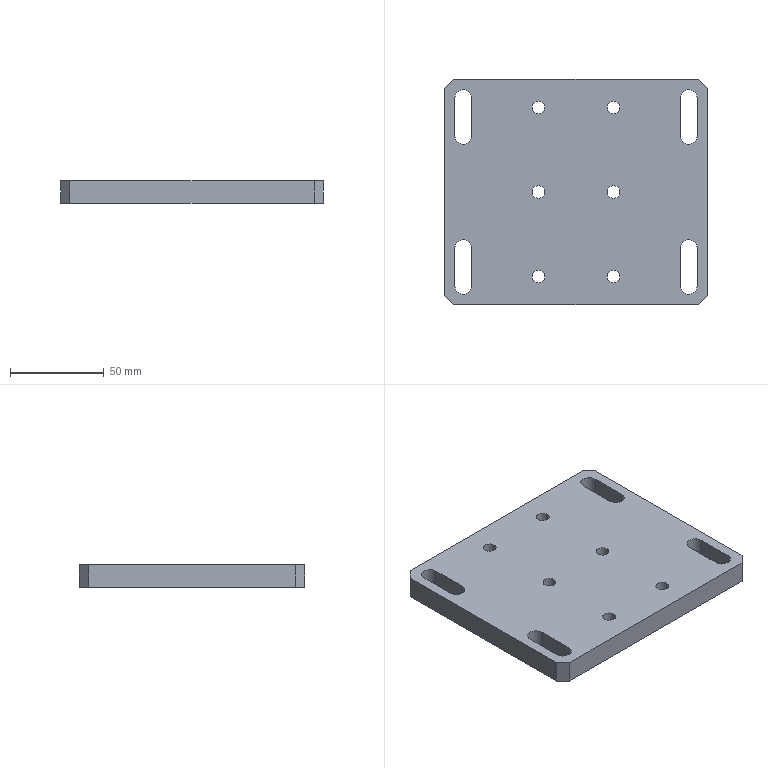Part | SolidWorks | features BaseBody 1 | 1 solid | 38 faces | box 140 x 120 x 12 mm | volume 186692 mm3 | cylinder 20 | plane 18 | commonest cylinder face diameters 6.8 x12 9 x8
STEP:
#1=CARTESIAN_POINT('',(16.6,-45.,0.));
#2=VERTEX_POINT('',#1);
#3=CARTESIAN_POINT('',(23.4,-45.,0.));
#4=VERTEX_POINT('',#3);
#5=CARTESIAN_POINT('',(20.,-45.,0.));
#6=DIRECTION('',(0.,0.,1.));
#7=DIRECTION('',(1.,0.,0.));
#8=AXIS2_PLACEMENT_3D('',#5,#6,#7);
#9=CIRCLE('',#8,3.4);
#10=EDGE_CURVE('',#2,#4,#9,.T.);
#11=ORIENTED_EDGE('',*,*,#10,.F.);
#12=CARTESIAN_POINT('',(16.6,-45.,12.));
#13=VERTEX_POINT('',#12);
#14=CARTESIAN_POINT('',(16.6,-45.,12.));
#15=DIRECTION('',(0.,0.,1.));
#16=VECTOR('',#15,1000.);
#17=LINE('',#14,#16);
#18=EDGE_CURVE('',#2,#13,#17,.T.);
#19=ORIENTED_EDGE('',*,*,#18,.T.);
#20=CARTESIAN_POINT('',(23.4,-45.,12.));
#21=VERTEX_POINT('',#20);
#22=CARTESIAN_POINT('',(20.,-45.,12.));
#23=DIRECTION('',(0.,0.,1.));
#24=DIRECTION('',(1.,0.,0.));
#25=AXIS2_PLACEMENT_3D('',#22,#23,#24);
#26=CIRCLE('',#25,3.4);
#27=EDGE_CURVE('',#13,#21,#26,.T.);
#28=ORIENTED_EDGE('',*,*,#27,.T.);
#29=CARTESIAN_POINT('',(23.4,-45.,12.));
#30=DIRECTION('',(0.,0.,1.));
#31=VECTOR('',#30,1000.);
#32=LINE('',#29,#31);
#33=EDGE_CURVE('',#4,#21,#32,.T.);
#34=ORIENTED_EDGE('',*,*,#33,.F.);
#35=EDGE_LOOP('',(#11,#19,#28,#34));
#36=FACE_OUTER_BOUND('',#35,.T.);
#37=CARTESIAN_POINT('',(20.,-45.,12.));
#38=DIRECTION('',(0.,0.,1.));
#39=DIRECTION('',(1.,0.,0.));
#40=AXIS2_PLACEMENT_3D('',#37,#38,#39);
#41=CYLINDRICAL_SURFACE('',#40,3.4);
#42=ADVANCED_FACE('',(#36),#41,.F.);
#43=CARTESIAN_POINT('',(-23.4,45.,0.));
#44=VERTEX_POINT('',#43);
#45=CARTESIAN_POINT('',(-16.6,45.,0.));
#46=VERTEX_POINT('',#45);
#47=CARTESIAN_POINT('',(-20.,45.,0.));
#48=DIRECTION('',(0.,0.,1.));
#49=DIRECTION('',(1.,0.,0.));
#50=AXIS2_PLACEMENT_3D('',#47,#48,#49);
#51=CIRCLE('',#50,3.4);
#52=EDGE_CURVE('',#44,#46,#51,.T.);
#53=ORIENTED_EDGE('',*,*,#52,.F.);
#54=CARTESIAN_POINT('',(-23.4,45.,12.));
#55=VERTEX_POINT('',#54);
#56=CARTESIAN_POINT('',(-23.4,45.,12.));
#57=DIRECTION('',(0.,0.,1.));
#58=VECTOR('',#57,1000.);
#59=LINE('',#56,#58);
#60=EDGE_CURVE('',#44,#55,#59,.T.);
#61=ORIENTED_EDGE('',*,*,#60,.T.);
#62=CARTESIAN_POINT('',(-16.6,45.,12.));
#63=VERTEX_POINT('',#62);
#64=CARTESIAN_POINT('',(-20.,45.,12.));
#65=DIRECTION('',(0.,0.,1.));
#66=DIRECTION('',(1.,0.,0.));
#67=AXIS2_PLACEMENT_3D('',#64,#65,#66);
#68=CIRCLE('',#67,3.4);
#69=EDGE_CURVE('',#55,#63,#68,.T.);
#70=ORIENTED_EDGE('',*,*,#69,.T.);
#71=CARTESIAN_POINT('',(-16.6,45.,12.));
#72=DIRECTION('',(0.,0.,1.));
#73=VECTOR('',#72,1000.);
#74=LINE('',#71,#73);
#75=EDGE_CURVE('',#46,#63,#74,.T.);
#76=ORIENTED_EDGE('',*,*,#75,.F.);
#77=EDGE_LOOP('',(#53,#61,#70,#76));
#78=FACE_OUTER_BOUND('',#77,.T.);
#79=CARTESIAN_POINT('',(-20.,45.,12.));
#80=DIRECTION('',(0.,0.,1.));
#81=DIRECTION('',(1.,0.,0.));
#82=AXIS2_PLACEMENT_3D('',#79,#80,#81);
#83=CYLINDRICAL_SURFACE('',#82,3.4);
#84=ADVANCED_FACE('',(#78),#83,.F.);
#85=CARTESIAN_POINT('',(-23.4,-45.,0.));
#86=VERTEX_POINT('',#85);
#87=CARTESIAN_POINT('',(-16.6,-45.,0.));
#88=VERTEX_POINT('',#87);
#89=CARTESIAN_POINT('',(-20.,-45.,0.));
#90=DIRECTION('',(0.,0.,1.));
#91=DIRECTION('',(1.,0.,0.));
#92=AXIS2_PLACEMENT_3D('',#89,#90,#91);
#93=CIRCLE('',#92,3.4);
#94=EDGE_CURVE('',#86,#88,#93,.T.);
#95=ORIENTED_EDGE('',*,*,#94,.F.);
#96=CARTESIAN_POINT('',(-23.4,-45.,12.));
#97=VERTEX_POINT('',#96);
#98=CARTESIAN_POINT('',(-23.4,-45.,12.));
#99=DIRECTION('',(0.,0.,1.));
#100=VECTOR('',#99,1000.);
#101=LINE('',#98,#100);
#102=EDGE_CURVE('',#86,#97,#101,.T.);
#103=ORIENTED_EDGE('',*,*,#102,.T.);
#104=CARTESIAN_POINT('',(-16.6,-45.,12.));
#105=VERTEX_POINT('',#104);
#106=CARTESIAN_POINT('',(-20.,-45.,12.));
#107=DIRECTION('',(0.,0.,1.));
#108=DIRECTION('',(1.,0.,0.));
#109=AXIS2_PLACEMENT_3D('',#106,#107,#108);
#110=CIRCLE('',#109,3.4);
#111=EDGE_CURVE('',#97,#105,#110,.T.);
#112=ORIENTED_EDGE('',*,*,#111,.T.);
#113=CARTESIAN_POINT('',(-16.6,-45.,12.));
#114=DIRECTION('',(0.,0.,1.));
#115=VECTOR('',#114,1000.);
#116=LINE('',#113,#115);
#117=EDGE_CURVE('',#88,#105,#116,.T.);
#118=ORIENTED_EDGE('',*,*,#117,.F.);
#119=EDGE_LOOP('',(#95,#103,#112,#118));
#120=FACE_OUTER_BOUND('',#119,.T.);
#121=CARTESIAN_POINT('',(-20.,-45.,12.));
#122=DIRECTION('',(0.,0.,1.));
#123=DIRECTION('',(1.,0.,0.));
#124=AXIS2_PLACEMENT_3D('',#121,#122,#123);
#125=CYLINDRICAL_SURFACE('',#124,3.4);
#126=ADVANCED_FACE('',(#120),#125,.F.);
#127=CARTESIAN_POINT('',(16.6,45.,0.));
#128=VERTEX_POINT('',#127);
#129=CARTESIAN_POINT('',(23.4,45.,0.));
#130=VERTEX_POINT('',#129);
#131=CARTESIAN_POINT('',(20.,45.,0.));
#132=DIRECTION('',(0.,0.,1.));
#133=DIRECTION('',(1.,0.,0.));
#134=AXIS2_PLACEMENT_3D('',#131,#132,#133);
#135=CIRCLE('',#134,3.4);
#136=EDGE_CURVE('',#128,#130,#135,.T.);
#137=ORIENTED_EDGE('',*,*,#136,.F.);
#138=CARTESIAN_POINT('',(16.6,45.,12.));
#139=VERTEX_POINT('',#138);
#140=CARTESIAN_POINT('',(16.6,45.,12.));
#141=DIRECTION('',(0.,0.,1.));
#142=VECTOR('',#141,1000.);
#143=LINE('',#140,#142);
#144=EDGE_CURVE('',#128,#139,#143,.T.);
#145=ORIENTED_EDGE('',*,*,#144,.T.);
#146=CARTESIAN_POINT('',(23.4,45.,12.));
#147=VERTEX_POINT('',#146);
#148=CARTESIAN_POINT('',(20.,45.,12.));
#149=DIRECTION('',(0.,0.,1.));
#150=DIRECTION('',(1.,0.,0.));
#151=AXIS2_PLACEMENT_3D('',#148,#149,#150);
#152=CIRCLE('',#151,3.4);
#153=EDGE_CURVE('',#139,#147,#152,.T.);
#154=ORIENTED_EDGE('',*,*,#153,.T.);
#155=CARTESIAN_POINT('',(23.4,45.,12.));
#156=DIRECTION('',(0.,0.,1.));
#157=VECTOR('',#156,1000.);
#158=LINE('',#155,#157);
#159=EDGE_CURVE('',#130,#147,#158,.T.);
#160=ORIENTED_EDGE('',*,*,#159,.F.);
#161=EDGE_LOOP('',(#137,#145,#154,#160));
#162=FACE_OUTER_BOUND('',#161,.T.);
#163=CARTESIAN_POINT('',(20.,45.,12.));
#164=DIRECTION('',(0.,0.,1.));
#165=DIRECTION('',(1.,0.,0.));
#166=AXIS2_PLACEMENT_3D('',#163,#164,#165);
#167=CYLINDRICAL_SURFACE('',#166,3.4);
#168=ADVANCED_FACE('',(#162),#167,.F.);
#169=CARTESIAN_POINT('',(-23.4,0.,0.));
#170=VERTEX_POINT('',#169);
#171=CARTESIAN_POINT('',(-16.6,0.,0.));
#172=VERTEX_POINT('',#171);
#173=CARTESIAN_POINT('',(-20.,0.,0.));
#174=DIRECTION('',(0.,0.,1.));
#175=DIRECTION('',(1.,0.,0.));
#176=AXIS2_PLACEMENT_3D('',#173,#174,#175);
#177=CIRCLE('',#176,3.4);
#178=EDGE_CURVE('',#170,#172,#177,.T.);
#179=ORIENTED_EDGE('',*,*,#178,.F.);
#180=CARTESIAN_POINT('',(-23.4,0.,12.));
#181=VERTEX_POINT('',#180);
#182=CARTESIAN_POINT('',(-23.4,0.,12.));
#183=DIRECTION('',(0.,0.,1.));
#184=VECTOR('',#183,1000.);
#185=LINE('',#182,#184);
#186=EDGE_CURVE('',#170,#181,#185,.T.);
#187=ORIENTED_EDGE('',*,*,#186,.T.);
#188=CARTESIAN_POINT('',(-16.6,0.,12.));
#189=VERTEX_POINT('',#188);
#190=CARTESIAN_POINT('',(-20.,0.,12.));
#191=DIRECTION('',(0.,0.,1.));
#192=DIRECTION('',(1.,0.,0.));
#193=AXIS2_PLACEMENT_3D('',#190,#191,#192);
#194=CIRCLE('',#193,3.4);
#195=EDGE_CURVE('',#181,#189,#194,.T.);
#196=ORIENTED_EDGE('',*,*,#195,.T.);
#197=CARTESIAN_POINT('',(-16.6,0.,12.));
#198=DIRECTION('',(0.,0.,1.));
#199=VECTOR('',#198,1000.);
#200=LINE('',#197,#199);
#201=EDGE_CURVE('',#172,#189,#200,.T.);
#202=ORIENTED_EDGE('',*,*,#201,.F.);
#203=EDGE_LOOP('',(#179,#187,#196,#202));
#204=FACE_OUTER_BOUND('',#203,.T.);
#205=CARTESIAN_POINT('',(-20.,0.,12.));
#206=DIRECTION('',(0.,0.,1.));
#207=DIRECTION('',(1.,0.,0.));
#208=AXIS2_PLACEMENT_3D('',#205,#206,#207);
#209=CYLINDRICAL_SURFACE('',#208,3.4);
#210=ADVANCED_FACE('',(#204),#209,.F.);
#211=CARTESIAN_POINT('',(16.6,0.,0.));
#212=VERTEX_POINT('',#211);
#213=CARTESIAN_POINT('',(23.4,0.,0.));
#214=VERTEX_POINT('',#213);
#215=CARTESIAN_POINT('',(20.,0.,0.));
#216=DIRECTION('',(0.,0.,1.));
#217=DIRECTION('',(1.,0.,0.));
#218=AXIS2_PLACEMENT_3D('',#215,#216,#217);
#219=CIRCLE('',#218,3.4);
#220=EDGE_CURVE('',#212,#214,#219,.T.);
#221=ORIENTED_EDGE('',*,*,#220,.F.);
#222=CARTESIAN_POINT('',(16.6,0.,12.));
#223=VERTEX_POINT('',#222);
#224=CARTESIAN_POINT('',(16.6,0.,12.));
#225=DIRECTION('',(0.,0.,1.));
#226=VECTOR('',#225,1000.);
#227=LINE('',#224,#226);
#228=EDGE_CURVE('',#212,#223,#227,.T.);
#229=ORIENTED_EDGE('',*,*,#228,.T.);
#230=CARTESIAN_POINT('',(23.4,0.,12.));
#231=VERTEX_POINT('',#230);
#232=CARTESIAN_POINT('',(20.,0.,12.));
#233=DIRECTION('',(0.,0.,1.));
#234=DIRECTION('',(1.,0.,0.));
#235=AXIS2_PLACEMENT_3D('',#232,#233,#234);
#236=CIRCLE('',#235,3.4);
#237=EDGE_CURVE('',#223,#231,#236,.T.);
#238=ORIENTED_EDGE('',*,*,#237,.T.);
#239=CARTESIAN_POINT('',(23.4,0.,12.));
#240=DIRECTION('',(0.,0.,1.));
#241=VECTOR('',#240,1000.);
#242=LINE('',#239,#241);
#243=EDGE_CURVE('',#214,#231,#242,.T.);
#244=ORIENTED_EDGE('',*,*,#243,.F.);
#245=EDGE_LOOP('',(#221,#229,#238,#244));
#246=FACE_OUTER_BOUND('',#245,.T.);
#247=CARTESIAN_POINT('',(20.,0.,12.));
#248=DIRECTION('',(0.,0.,1.));
#249=DIRECTION('',(1.,0.,0.));
#250=AXIS2_PLACEMENT_3D('',#247,#248,#249);
#251=CYLINDRICAL_SURFACE('',#250,3.4);
#252=ADVANCED_FACE('',(#246),#251,.F.);
#253=CARTESIAN_POINT('',(20.,-45.,12.));
#254=DIRECTION('',(0.,0.,1.));
#255=DIRECTION('',(1.,0.,0.));
#256=AXIS2_PLACEMENT_3D('',#253,#254,#255);
#257=CIRCLE('',#256,3.4);
#258=EDGE_CURVE('',#21,#13,#257,.T.);
#259=ORIENTED_EDGE('',*,*,#258,.F.);
#260=ORIENTED_EDGE('',*,*,#27,.F.);
#261=EDGE_LOOP('',(#259,#260));
#262=FACE_BOUND('',#261,.T.);
#263=CARTESIAN_POINT('',(-20.,45.,12.));
#264=DIRECTION('',(0.,0.,1.));
#265=DIRECTION('',(1.,0.,0.));
#266=AXIS2_PLACEMENT_3D('',#263,#264,#265);
#267=CIRCLE('',#266,3.4);
#268=EDGE_CURVE('',#63,#55,#267,.T.);
#269=ORIENTED_EDGE('',*,*,#268,.F.);
#270=ORIENTED_EDGE('',*,*,#69,.F.);
#271=EDGE_LOOP('',(#269,#270));
#272=FACE_BOUND('',#271,.T.);
#273=CARTESIAN_POINT('',(-20.,-45.,12.));
#274=DIRECTION('',(0.,0.,1.));
#275=DIRECTION('',(1.,0.,0.));
#276=AXIS2_PLACEMENT_3D('',#273,#274,#275);
#277=CIRCLE('',#276,3.4);
#278=EDGE_CURVE('',#105,#97,#277,.T.);
#279=ORIENTED_EDGE('',*,*,#278,.F.);
#280=ORIENTED_EDGE('',*,*,#111,.F.);
#281=EDGE_LOOP('',(#279,#280));
#282=FACE_BOUND('',#281,.T.);
#283=CARTESIAN_POINT('',(20.,45.,12.));
#284=DIRECTION('',(0.,0.,1.));
#285=DIRECTION('',(1.,0.,0.));
#286=AXIS2_PLACEMENT_3D('',#283,#284,#285);
#287=CIRCLE('',#286,3.4);
#288=EDGE_CURVE('',#147,#139,#287,.T.);
#289=ORIENTED_EDGE('',*,*,#288,.F.);
#290=ORIENTED_EDGE('',*,*,#153,.F.);
#291=EDGE_LOOP('',(#289,#290));
#292=FACE_BOUND('',#291,.T.);
#293=CARTESIAN_POINT('',(-20.,0.,12.));
#294=DIRECTION('',(0.,0.,1.));
#295=DIRECTION('',(1.,0.,0.));
#296=AXIS2_PLACEMENT_3D('',#293,#294,#295);
#297=CIRCLE('',#296,3.4);
#298=EDGE_CURVE('',#189,#181,#297,.T.);
#299=ORIENTED_EDGE('',*,*,#298,.F.);
#300=ORIENTED_EDGE('',*,*,#195,.F.);
#301=EDGE_LOOP('',(#299,#300));
#302=FACE_BOUND('',#301,.T.);
#303=CARTESIAN_POINT('',(55.5,-50.,12.));
#304=VERTEX_POINT('',#303);
#305=CARTESIAN_POINT('',(64.5,-50.,12.));
#306=VERTEX_POINT('',#305);
#307=CARTESIAN_POINT('',(60.,-50.,12.));
#308=DIRECTION('',(0.,0.,1.));
#309=DIRECTION('',(1.,0.,0.));
#310=AXIS2_PLACEMENT_3D('',#307,#308,#309);
#311=CIRCLE('',#310,4.5);
#312=EDGE_CURVE('',#304,#306,#311,.T.);
#313=ORIENTED_EDGE('',*,*,#312,.F.);
#314=CARTESIAN_POINT('',(55.5,-30.,12.));
#315=VERTEX_POINT('',#314);
#316=CARTESIAN_POINT('',(55.5,-50.,12.));
#317=DIRECTION('',(0.,-1.,0.));
#318=VECTOR('',#317,1000.);
#319=LINE('',#316,#318);
#320=EDGE_CURVE('',#315,#304,#319,.T.);
#321=ORIENTED_EDGE('',*,*,#320,.F.);
#322=CARTESIAN_POINT('',(64.5,-30.,12.));
#323=VERTEX_POINT('',#322);
#324=CARTESIAN_POINT('',(60.,-30.,12.));
#325=DIRECTION('',(0.,0.,1.));
#326=DIRECTION('',(1.,0.,0.));
#327=AXIS2_PLACEMENT_3D('',#324,#325,#326);
#328=CIRCLE('',#327,4.5);
#329=EDGE_CURVE('',#323,#315,#328,.T.);
#330=ORIENTED_EDGE('',*,*,#329,.F.);
#331=CARTESIAN_POINT('',(64.5,-50.,12.));
#332=DIRECTION('',(0.,1.,0.));
#333=VECTOR('',#332,1000.);
#334=LINE('',#331,#333);
#335=EDGE_CURVE('',#306,#323,#334,.T.);
#336=ORIENTED_EDGE('',*,*,#335,.F.);
#337=EDGE_LOOP('',(#313,#321,#330,#336));
#338=FACE_BOUND('',#337,.T.);
#339=CARTESIAN_POINT('',(-55.5,50.,12.));
#340=VERTEX_POINT('',#339);
#341=CARTESIAN_POINT('',(-64.5,50.,12.));
#342=VERTEX_POINT('',#341);
#343=CARTESIAN_POINT('',(-60.,50.,12.));
#344=DIRECTION('',(0.,0.,1.));
#345=DIRECTION('',(1.,0.,0.));
#346=AXIS2_PLACEMENT_3D('',#343,#344,#345);
#347=CIRCLE('',#346,4.5);
#348=EDGE_CURVE('',#340,#342,#347,.T.);
#349=ORIENTED_EDGE('',*,*,#348,.F.);
#350=CARTESIAN_POINT('',(-55.5,30.,12.));
#351=VERTEX_POINT('',#350);
#352=CARTESIAN_POINT('',(-55.5,50.,12.));
#353=DIRECTION('',(0.,1.,0.));
#354=VECTOR('',#353,1000.);
#355=LINE('',#352,#354);
#356=EDGE_CURVE('',#351,#340,#355,.T.);
#357=ORIENTED_EDGE('',*,*,#356,.F.);
#358=CARTESIAN_POINT('',(-64.5,30.,12.));
#359=VERTEX_POINT('',#358);
#360=CARTESIAN_POINT('',(-60.,30.,12.));
#361=DIRECTION('',(0.,0.,1.));
#362=DIRECTION('',(1.,0.,0.));
#363=AXIS2_PLACEMENT_3D('',#360,#361,#362);
#364=CIRCLE('',#363,4.5);
#365=EDGE_CURVE('',#359,#351,#364,.T.);
#366=ORIENTED_EDGE('',*,*,#365,.F.);
#367=CARTESIAN_POINT('',(-64.5,50.,12.));
#368=DIRECTION('',(0.,-1.,0.));
#369=VECTOR('',#368,1000.);
#370=LINE('',#367,#369);
#371=EDGE_CURVE('',#342,#359,#370,.T.);
#372=ORIENTED_EDGE('',*,*,#371,.F.);
#373=EDGE_LOOP('',(#349,#357,#366,#372));
#374=FACE_BOUND('',#373,.T.);
#375=CARTESIAN_POINT('',(65.,60.,12.));
#376=VERTEX_POINT('',#375);
#377=CARTESIAN_POINT('',(-65.,60.,12.));
#378=VERTEX_POINT('',#377);
#379=CARTESIAN_POINT('',(-65.,60.,12.));
#380=DIRECTION('',(-1.,0.,0.));
#381=VECTOR('',#380,1000.);
#382=LINE('',#379,#381);
#383=EDGE_CURVE('',#376,#378,#382,.T.);
#384=ORIENTED_EDGE('',*,*,#383,.T.);
#385=CARTESIAN_POINT('',(-70.,55.,12.));
#386=VERTEX_POINT('',#385);
#387=CARTESIAN_POINT('',(-70.,55.,12.));
#388=DIRECTION('',(-0.7071,-0.7071,0.));
#389=VECTOR('',#388,1000.);
#390=LINE('',#387,#389);
#391=EDGE_CURVE('',#378,#386,#390,.T.);
#392=ORIENTED_EDGE('',*,*,#391,.T.);
#393=CARTESIAN_POINT('',(-70.,-55.,12.));
#394=VERTEX_POINT('',#393);
#395=CARTESIAN_POINT('',(-70.,55.,12.));
#396=DIRECTION('',(0.,-1.,0.));
#397=VECTOR('',#396,1000.);
#398=LINE('',#395,#397);
#399=EDGE_CURVE('',#386,#394,#398,.T.);
#400=ORIENTED_EDGE('',*,*,#399,.T.);
#401=CARTESIAN_POINT('',(-65.,-60.,12.));
#402=VERTEX_POINT('',#401);
#403=CARTESIAN_POINT('',(-70.,-55.,12.));
#404=DIRECTION('',(0.7071,-0.7071,0.));
#405=VECTOR('',#404,1000.);
#406=LINE('',#403,#405);
#407=EDGE_CURVE('',#394,#402,#406,.T.);
#408=ORIENTED_EDGE('',*,*,#407,.T.);
#409=CARTESIAN_POINT('',(65.,-60.,12.));
#410=VERTEX_POINT('',#409);
#411=CARTESIAN_POINT('',(-65.,-60.,12.));
#412=DIRECTION('',(1.,0.,0.));
#413=VECTOR('',#412,1000.);
#414=LINE('',#411,#413);
#415=EDGE_CURVE('',#402,#410,#414,.T.);
#416=ORIENTED_EDGE('',*,*,#415,.T.);
#417=CARTESIAN_POINT('',(70.,-55.,12.));
#418=VERTEX_POINT('',#417);
#419=CARTESIAN_POINT('',(65.,-60.,12.));
#420=DIRECTION('',(0.7071,0.7071,0.));
#421=VECTOR('',#420,1000.);
#422=LINE('',#419,#421);
#423=EDGE_CURVE('',#410,#418,#422,.T.);
#424=ORIENTED_EDGE('',*,*,#423,.T.);
#425=CARTESIAN_POINT('',(70.,55.,12.));
#426=VERTEX_POINT('',#425);
#427=CARTESIAN_POINT('',(70.,55.,12.));
#428=DIRECTION('',(0.,1.,0.));
#429=VECTOR('',#428,1000.);
#430=LINE('',#427,#429);
#431=EDGE_CURVE('',#418,#426,#430,.T.);
#432=ORIENTED_EDGE('',*,*,#431,.T.);
#433=CARTESIAN_POINT('',(65.,60.,12.));
#434=DIRECTION('',(-0.7071,0.7071,0.));
#435=VECTOR('',#434,1000.);
#436=LINE('',#433,#435);
#437=EDGE_CURVE('',#426,#376,#436,.T.);
#438=ORIENTED_EDGE('',*,*,#437,.T.);
#439=EDGE_LOOP('',(#384,#392,#400,#408,#416,#424,#432,#438));
#440=FACE_OUTER_BOUND('',#439,.T.);
#441=CARTESIAN_POINT('',(64.5,50.,12.));
#442=VERTEX_POINT('',#441);
#443=CARTESIAN_POINT('',(55.5,50.,12.));
#444=VERTEX_POINT('',#443);
#445=CARTESIAN_POINT('',(60.,50.,12.));
#446=DIRECTION('',(0.,0.,1.));
#447=DIRECTION('',(1.,0.,0.));
#448=AXIS2_PLACEMENT_3D('',#445,#446,#447);
#449=CIRCLE('',#448,4.5);
#450=EDGE_CURVE('',#442,#444,#449,.T.);
#451=ORIENTED_EDGE('',*,*,#450,.F.);
#452=CARTESIAN_POINT('',(64.5,30.,12.));
#453=VERTEX_POINT('',#452);
#454=CARTESIAN_POINT('',(64.5,50.,12.));
#455=DIRECTION('',(0.,1.,0.));
#456=VECTOR('',#455,1000.);
#457=LINE('',#454,#456);
#458=EDGE_CURVE('',#453,#442,#457,.T.);
#459=ORIENTED_EDGE('',*,*,#458,.F.);
#460=CARTESIAN_POINT('',(55.5,30.,12.));
#461=VERTEX_POINT('',#460);
#462=CARTESIAN_POINT('',(60.,30.,12.));
#463=DIRECTION('',(0.,0.,1.));
#464=DIRECTION('',(1.,0.,0.));
#465=AXIS2_PLACEMENT_3D('',#462,#463,#464);
#466=CIRCLE('',#465,4.5);
#467=EDGE_CURVE('',#461,#453,#466,.T.);
#468=ORIENTED_EDGE('',*,*,#467,.F.);
#469=CARTESIAN_POINT('',(55.5,50.,12.));
#470=DIRECTION('',(0.,-1.,0.));
#471=VECTOR('',#470,1000.);
#472=LINE('',#469,#471);
#473=EDGE_CURVE('',#444,#461,#472,.T.);
#474=ORIENTED_EDGE('',*,*,#473,.F.);
#475=EDGE_LOOP('',(#451,#459,#468,#474));
#476=FACE_BOUND('',#475,.T.);
#477=CARTESIAN_POINT('',(-64.5,-50.,12.));
#478=VERTEX_POINT('',#477);
#479=CARTESIAN_POINT('',(-55.5,-50.,12.));
#480=VERTEX_POINT('',#479);
#481=CARTESIAN_POINT('',(-60.,-50.,12.));
#482=DIRECTION('',(0.,0.,1.));
#483=DIRECTION('',(1.,0.,0.));
#484=AXIS2_PLACEMENT_3D('',#481,#482,#483);
#485=CIRCLE('',#484,4.5);
#486=EDGE_CURVE('',#478,#480,#485,.T.);
#487=ORIENTED_EDGE('',*,*,#486,.F.);
#488=CARTESIAN_POINT('',(-64.5,-30.,12.));
#489=VERTEX_POINT('',#488);
#490=CARTESIAN_POINT('',(-64.5,-50.,12.));
#491=DIRECTION('',(0.,-1.,0.));
#492=VECTOR('',#491,1000.);
#493=LINE('',#490,#492);
#494=EDGE_CURVE('',#489,#478,#493,.T.);
#495=ORIENTED_EDGE('',*,*,#494,.F.);
#496=CARTESIAN_POINT('',(-55.5,-30.,12.));
#497=VERTEX_POINT('',#496);
#498=CARTESIAN_POINT('',(-60.,-30.,12.));
#499=DIRECTION('',(0.,0.,1.));
#500=DIRECTION('',(1.,0.,0.));
#501=AXIS2_PLACEMENT_3D('',#498,#499,#500);
#502=CIRCLE('',#501,4.5);
#503=EDGE_CURVE('',#497,#489,#502,.T.);
#504=ORIENTED_EDGE('',*,*,#503,.F.);
#505=CARTESIAN_POINT('',(-55.5,-50.,12.));
#506=DIRECTION('',(0.,1.,0.));
#507=VECTOR('',#506,1000.);
#508=LINE('',#505,#507);
#509=EDGE_CURVE('',#480,#497,#508,.T.);
#510=ORIENTED_EDGE('',*,*,#509,.F.);
#511=EDGE_LOOP('',(#487,#495,#504,#510));
#512=FACE_BOUND('',#511,.T.);
#513=CARTESIAN_POINT('',(20.,0.,12.));
#514=DIRECTION('',(0.,0.,1.));
#515=DIRECTION('',(1.,0.,0.));
#516=AXIS2_PLACEMENT_3D('',#513,#514,#515);
#517=CIRCLE('',#516,3.4);
#518=EDGE_CURVE('',#231,#223,#517,.T.);
#519=ORIENTED_EDGE('',*,*,#518,.F.);
#520=ORIENTED_EDGE('',*,*,#237,.F.);
#521=EDGE_LOOP('',(#519,#520));
#522=FACE_BOUND('',#521,.T.);
#523=CARTESIAN_POINT('',(0.,0.,12.));
#524=DIRECTION('',(0.,0.,-1.));
#525=DIRECTION('',(-1.,0.,0.));
#526=AXIS2_PLACEMENT_3D('',#523,#524,#525);
#527=PLANE('',#526);
#528=ADVANCED_FACE('',(#262,#272,#282,#292,#302,#338,#374,#440,#476,#512,#522),#527,.F.);
#529=CARTESIAN_POINT('',(20.,-45.,0.));
#530=DIRECTION('',(0.,0.,1.));
#531=DIRECTION('',(1.,0.,0.));
#532=AXIS2_PLACEMENT_3D('',#529,#530,#531);
#533=CIRCLE('',#532,3.4);
#534=EDGE_CURVE('',#4,#2,#533,.T.);
#535=ORIENTED_EDGE('',*,*,#534,.T.);
#536=ORIENTED_EDGE('',*,*,#10,.T.);
#537=EDGE_LOOP('',(#535,#536));
#538=FACE_BOUND('',#537,.T.);
#539=CARTESIAN_POINT('',(-20.,45.,0.));
#540=DIRECTION('',(0.,0.,1.));
#541=DIRECTION('',(1.,0.,0.));
#542=AXIS2_PLACEMENT_3D('',#539,#540,#541);
#543=CIRCLE('',#542,3.4);
#544=EDGE_CURVE('',#46,#44,#543,.T.);
#545=ORIENTED_EDGE('',*,*,#544,.T.);
#546=ORIENTED_EDGE('',*,*,#52,.T.);
#547=EDGE_LOOP('',(#545,#546));
#548=FACE_BOUND('',#547,.T.);
#549=CARTESIAN_POINT('',(-20.,-45.,0.));
#550=DIRECTION('',(0.,0.,1.));
#551=DIRECTION('',(1.,0.,0.));
#552=AXIS2_PLACEMENT_3D('',#549,#550,#551);
#553=CIRCLE('',#552,3.4);
#554=EDGE_CURVE('',#88,#86,#553,.T.);
#555=ORIENTED_EDGE('',*,*,#554,.T.);
#556=ORIENTED_EDGE('',*,*,#94,.T.);
#557=EDGE_LOOP('',(#555,#556));
#558=FACE_BOUND('',#557,.T.);
#559=CARTESIAN_POINT('',(20.,45.,0.));
#560=DIRECTION('',(0.,0.,1.));
#561=DIRECTION('',(1.,0.,0.));
#562=AXIS2_PLACEMENT_3D('',#559,#560,#561);
#563=CIRCLE('',#562,3.4);
#564=EDGE_CURVE('',#130,#128,#563,.T.);
#565=ORIENTED_EDGE('',*,*,#564,.T.);
#566=ORIENTED_EDGE('',*,*,#136,.T.);
#567=EDGE_LOOP('',(#565,#566));
#568=FACE_BOUND('',#567,.T.);
#569=CARTESIAN_POINT('',(-20.,0.,0.));
#570=DIRECTION('',(0.,0.,1.));
#571=DIRECTION('',(1.,0.,0.));
#572=AXIS2_PLACEMENT_3D('',#569,#570,#571);
#573=CIRCLE('',#572,3.4);
#574=EDGE_CURVE('',#172,#170,#573,.T.);
#575=ORIENTED_EDGE('',*,*,#574,.T.);
#576=ORIENTED_EDGE('',*,*,#178,.T.);
#577=EDGE_LOOP('',(#575,#576));
#578=FACE_BOUND('',#577,.T.);
#579=CARTESIAN_POINT('',(-64.5,-30.,0.));
#580=VERTEX_POINT('',#579);
#581=CARTESIAN_POINT('',(-64.5,-50.,0.));
#582=VERTEX_POINT('',#581);
#583=CARTESIAN_POINT('',(-64.5,-50.,0.));
#584=DIRECTION('',(0.,-1.,0.));
#585=VECTOR('',#584,1000.);
#586=LINE('',#583,#585);
#587=EDGE_CURVE('',#580,#582,#586,.T.);
#588=ORIENTED_EDGE('',*,*,#587,.T.);
#589=CARTESIAN_POINT('',(-55.5,-50.,0.));
#590=VERTEX_POINT('',#589);
#591=CARTESIAN_POINT('',(-60.,-50.,0.));
#592=DIRECTION('',(0.,0.,1.));
#593=DIRECTION('',(1.,0.,0.));
#594=AXIS2_PLACEMENT_3D('',#591,#592,#593);
#595=CIRCLE('',#594,4.5);
#596=EDGE_CURVE('',#582,#590,#595,.T.);
#597=ORIENTED_EDGE('',*,*,#596,.T.);
#598=CARTESIAN_POINT('',(-55.5,-30.,0.));
#599=VERTEX_POINT('',#598);
#600=CARTESIAN_POINT('',(-55.5,-50.,0.));
#601=DIRECTION('',(0.,1.,0.));
#602=VECTOR('',#601,1000.);
#603=LINE('',#600,#602);
#604=EDGE_CURVE('',#590,#599,#603,.T.);
#605=ORIENTED_EDGE('',*,*,#604,.T.);
#606=CARTESIAN_POINT('',(-60.,-30.,0.));
#607=DIRECTION('',(0.,0.,1.));
#608=DIRECTION('',(1.,0.,0.));
#609=AXIS2_PLACEMENT_3D('',#606,#607,#608);
#610=CIRCLE('',#609,4.5);
#611=EDGE_CURVE('',#599,#580,#610,.T.);
#612=ORIENTED_EDGE('',*,*,#611,.T.);
#613=EDGE_LOOP('',(#588,#597,#605,#612));
#614=FACE_BOUND('',#613,.T.);
#615=CARTESIAN_POINT('',(55.5,-30.,0.));
#616=VERTEX_POINT('',#615);
#617=CARTESIAN_POINT('',(55.5,-50.,0.));
#618=VERTEX_POINT('',#617);
#619=CARTESIAN_POINT('',(55.5,-50.,0.));
#620=DIRECTION('',(0.,-1.,0.));
#621=VECTOR('',#620,1000.);
#622=LINE('',#619,#621);
#623=EDGE_CURVE('',#616,#618,#622,.T.);
#624=ORIENTED_EDGE('',*,*,#623,.T.);
#625=CARTESIAN_POINT('',(64.5,-50.,0.));
#626=VERTEX_POINT('',#625);
#627=CARTESIAN_POINT('',(60.,-50.,0.));
#628=DIRECTION('',(0.,0.,1.));
#629=DIRECTION('',(1.,0.,0.));
#630=AXIS2_PLACEMENT_3D('',#627,#628,#629);
#631=CIRCLE('',#630,4.5);
#632=EDGE_CURVE('',#618,#626,#631,.T.);
#633=ORIENTED_EDGE('',*,*,#632,.T.);
#634=CARTESIAN_POINT('',(64.5,-30.,0.));
#635=VERTEX_POINT('',#634);
#636=CARTESIAN_POINT('',(64.5,-50.,0.));
#637=DIRECTION('',(0.,1.,0.));
#638=VECTOR('',#637,1000.);
#639=LINE('',#636,#638);
#640=EDGE_CURVE('',#626,#635,#639,.T.);
#641=ORIENTED_EDGE('',*,*,#640,.T.);
#642=CARTESIAN_POINT('',(60.,-30.,0.));
#643=DIRECTION('',(0.,0.,1.));
#644=DIRECTION('',(1.,0.,0.));
#645=AXIS2_PLACEMENT_3D('',#642,#643,#644);
#646=CIRCLE('',#645,4.5);
#647=EDGE_CURVE('',#635,#616,#646,.T.);
#648=ORIENTED_EDGE('',*,*,#647,.T.);
#649=EDGE_LOOP('',(#624,#633,#641,#648));
#650=FACE_BOUND('',#649,.T.);
#651=CARTESIAN_POINT('',(64.5,30.,0.));
#652=VERTEX_POINT('',#651);
#653=CARTESIAN_POINT('',(64.5,50.,0.));
#654=VERTEX_POINT('',#653);
#655=CARTESIAN_POINT('',(64.5,50.,0.));
#656=DIRECTION('',(0.,1.,0.));
#657=VECTOR('',#656,1000.);
#658=LINE('',#655,#657);
#659=EDGE_CURVE('',#652,#654,#658,.T.);
#660=ORIENTED_EDGE('',*,*,#659,.T.);
#661=CARTESIAN_POINT('',(55.5,50.,0.));
#662=VERTEX_POINT('',#661);
#663=CARTESIAN_POINT('',(60.,50.,0.));
#664=DIRECTION('',(0.,0.,1.));
#665=DIRECTION('',(1.,0.,0.));
#666=AXIS2_PLACEMENT_3D('',#663,#664,#665);
#667=CIRCLE('',#666,4.5);
#668=EDGE_CURVE('',#654,#662,#667,.T.);
#669=ORIENTED_EDGE('',*,*,#668,.T.);
#670=CARTESIAN_POINT('',(55.5,30.,0.));
#671=VERTEX_POINT('',#670);
#672=CARTESIAN_POINT('',(55.5,50.,0.));
#673=DIRECTION('',(0.,-1.,0.));
#674=VECTOR('',#673,1000.);
#675=LINE('',#672,#674);
#676=EDGE_CURVE('',#662,#671,#675,.T.);
#677=ORIENTED_EDGE('',*,*,#676,.T.);
#678=CARTESIAN_POINT('',(60.,30.,0.));
#679=DIRECTION('',(0.,0.,1.));
#680=DIRECTION('',(1.,0.,0.));
#681=AXIS2_PLACEMENT_3D('',#678,#679,#680);
#682=CIRCLE('',#681,4.5);
#683=EDGE_CURVE('',#671,#652,#682,.T.);
#684=ORIENTED_EDGE('',*,*,#683,.T.);
#685=EDGE_LOOP('',(#660,#669,#677,#684));
#686=FACE_BOUND('',#685,.T.);
#687=CARTESIAN_POINT('',(-55.5,30.,0.));
#688=VERTEX_POINT('',#687);
#689=CARTESIAN_POINT('',(-55.5,50.,0.));
#690=VERTEX_POINT('',#689);
#691=CARTESIAN_POINT('',(-55.5,50.,0.));
#692=DIRECTION('',(0.,1.,0.));
#693=VECTOR('',#692,1000.);
#694=LINE('',#691,#693);
#695=EDGE_CURVE('',#688,#690,#694,.T.);
#696=ORIENTED_EDGE('',*,*,#695,.T.);
#697=CARTESIAN_POINT('',(-64.5,50.,0.));
#698=VERTEX_POINT('',#697);
#699=CARTESIAN_POINT('',(-60.,50.,0.));
#700=DIRECTION('',(0.,0.,1.));
#701=DIRECTION('',(1.,0.,0.));
#702=AXIS2_PLACEMENT_3D('',#699,#700,#701);
#703=CIRCLE('',#702,4.5);
#704=EDGE_CURVE('',#690,#698,#703,.T.);
#705=ORIENTED_EDGE('',*,*,#704,.T.);
#706=CARTESIAN_POINT('',(-64.5,30.,0.));
#707=VERTEX_POINT('',#706);
#708=CARTESIAN_POINT('',(-64.5,50.,0.));
#709=DIRECTION('',(0.,-1.,0.));
#710=VECTOR('',#709,1000.);
#711=LINE('',#708,#710);
#712=EDGE_CURVE('',#698,#707,#711,.T.);
#713=ORIENTED_EDGE('',*,*,#712,.T.);
#714=CARTESIAN_POINT('',(-60.,30.,0.));
#715=DIRECTION('',(0.,0.,1.));
#716=DIRECTION('',(1.,0.,0.));
#717=AXIS2_PLACEMENT_3D('',#714,#715,#716);
#718=CIRCLE('',#717,4.5);
#719=EDGE_CURVE('',#707,#688,#718,.T.);
#720=ORIENTED_EDGE('',*,*,#719,.T.);
#721=EDGE_LOOP('',(#696,#705,#713,#720));
#722=FACE_BOUND('',#721,.T.);
#723=CARTESIAN_POINT('',(65.,60.,0.));
#724=VERTEX_POINT('',#723);
#725=CARTESIAN_POINT('',(-65.,60.,0.));
#726=VERTEX_POINT('',#725);
#727=CARTESIAN_POINT('',(-65.,60.,0.));
#728=DIRECTION('',(-1.,0.,0.));
#729=VECTOR('',#728,1000.);
#730=LINE('',#727,#729);
#731=EDGE_CURVE('',#724,#726,#730,.T.);
#732=ORIENTED_EDGE('',*,*,#731,.F.);
#733=CARTESIAN_POINT('',(70.,55.,0.));
#734=VERTEX_POINT('',#733);
#735=CARTESIAN_POINT('',(65.,60.,0.));
#736=DIRECTION('',(-0.7071,0.7071,0.));
#737=VECTOR('',#736,1000.);
#738=LINE('',#735,#737);
#739=EDGE_CURVE('',#734,#724,#738,.T.);
#740=ORIENTED_EDGE('',*,*,#739,.F.);
#741=CARTESIAN_POINT('',(70.,-55.,0.));
#742=VERTEX_POINT('',#741);
#743=CARTESIAN_POINT('',(70.,55.,0.));
#744=DIRECTION('',(0.,1.,0.));
#745=VECTOR('',#744,1000.);
#746=LINE('',#743,#745);
#747=EDGE_CURVE('',#742,#734,#746,.T.);
#748=ORIENTED_EDGE('',*,*,#747,.F.);
#749=CARTESIAN_POINT('',(65.,-60.,0.));
#750=VERTEX_POINT('',#749);
#751=CARTESIAN_POINT('',(65.,-60.,0.));
#752=DIRECTION('',(0.7071,0.7071,0.));
#753=VECTOR('',#752,1000.);
#754=LINE('',#751,#753);
#755=EDGE_CURVE('',#750,#742,#754,.T.);
#756=ORIENTED_EDGE('',*,*,#755,.F.);
#757=CARTESIAN_POINT('',(-65.,-60.,0.));
#758=VERTEX_POINT('',#757);
#759=CARTESIAN_POINT('',(-65.,-60.,0.));
#760=DIRECTION('',(1.,0.,0.));
#761=VECTOR('',#760,1000.);
#762=LINE('',#759,#761);
#763=EDGE_CURVE('',#758,#750,#762,.T.);
#764=ORIENTED_EDGE('',*,*,#763,.F.);
#765=CARTESIAN_POINT('',(-70.,-55.,0.));
#766=VERTEX_POINT('',#765);
#767=CARTESIAN_POINT('',(-70.,-55.,0.));
#768=DIRECTION('',(0.7071,-0.7071,0.));
#769=VECTOR('',#768,1000.);
#770=LINE('',#767,#769);
#771=EDGE_CURVE('',#766,#758,#770,.T.);
#772=ORIENTED_EDGE('',*,*,#771,.F.);
#773=CARTESIAN_POINT('',(-70.,55.,0.));
#774=VERTEX_POINT('',#773);
#775=CARTESIAN_POINT('',(-70.,55.,0.));
#776=DIRECTION('',(0.,-1.,0.));
#777=VECTOR('',#776,1000.);
#778=LINE('',#775,#777);
#779=EDGE_CURVE('',#774,#766,#778,.T.);
#780=ORIENTED_EDGE('',*,*,#779,.F.);
#781=CARTESIAN_POINT('',(-70.,55.,0.));
#782=DIRECTION('',(-0.7071,-0.7071,0.));
#783=VECTOR('',#782,1000.);
#784=LINE('',#781,#783);
#785=EDGE_CURVE('',#726,#774,#784,.T.);
#786=ORIENTED_EDGE('',*,*,#785,.F.);
#787=EDGE_LOOP('',(#732,#740,#748,#756,#764,#772,#780,#786));
#788=FACE_OUTER_BOUND('',#787,.T.);
#789=CARTESIAN_POINT('',(20.,0.,0.));
#790=DIRECTION('',(0.,0.,1.));
#791=DIRECTION('',(1.,0.,0.));
#792=AXIS2_PLACEMENT_3D('',#789,#790,#791);
#793=CIRCLE('',#792,3.4);
#794=EDGE_CURVE('',#214,#212,#793,.T.);
#795=ORIENTED_EDGE('',*,*,#794,.T.);
#796=ORIENTED_EDGE('',*,*,#220,.T.);
#797=EDGE_LOOP('',(#795,#796));
#798=FACE_BOUND('',#797,.T.);
#799=CARTESIAN_POINT('',(0.,0.,0.));
#800=DIRECTION('',(0.,0.,-1.));
#801=DIRECTION('',(-1.,0.,0.));
#802=AXIS2_PLACEMENT_3D('',#799,#800,#801);
#803=PLANE('',#802);
#804=ADVANCED_FACE('',(#538,#548,#558,#568,#578,#614,#650,#686,#722,#788,#798),#803,.T.);
#805=ORIENTED_EDGE('',*,*,#731,.T.);
#806=CARTESIAN_POINT('',(-65.,60.,12.));
#807=DIRECTION('',(0.,0.,-1.));
#808=VECTOR('',#807,1000.);
#809=LINE('',#806,#808);
#810=EDGE_CURVE('',#378,#726,#809,.T.);
#811=ORIENTED_EDGE('',*,*,#810,.F.);
#812=ORIENTED_EDGE('',*,*,#383,.F.);
#813=CARTESIAN_POINT('',(65.,60.,12.));
#814=DIRECTION('',(0.,0.,-1.));
#815=VECTOR('',#814,1000.);
#816=LINE('',#813,#815);
#817=EDGE_CURVE('',#376,#724,#816,.T.);
#818=ORIENTED_EDGE('',*,*,#817,.T.);
#819=EDGE_LOOP('',(#805,#811,#812,#818));
#820=FACE_OUTER_BOUND('',#819,.T.);
#821=CARTESIAN_POINT('',(-65.,60.,12.));
#822=DIRECTION('',(0.,-1.,0.));
#823=DIRECTION('',(0.,0.,-1.));
#824=AXIS2_PLACEMENT_3D('',#821,#822,#823);
#825=PLANE('',#824);
#826=ADVANCED_FACE('',(#820),#825,.F.);
#827=ORIENTED_EDGE('',*,*,#785,.T.);
#828=CARTESIAN_POINT('',(-70.,55.,12.));
#829=DIRECTION('',(0.,0.,-1.));
#830=VECTOR('',#829,1000.);
#831=LINE('',#828,#830);
#832=EDGE_CURVE('',#386,#774,#831,.T.);
#833=ORIENTED_EDGE('',*,*,#832,.F.);
#834=ORIENTED_EDGE('',*,*,#391,.F.);
#835=ORIENTED_EDGE('',*,*,#810,.T.);
#836=EDGE_LOOP('',(#827,#833,#834,#835));
#837=FACE_OUTER_BOUND('',#836,.T.);
#838=CARTESIAN_POINT('',(-70.,55.,12.));
#839=DIRECTION('',(0.7071,-0.7071,0.));
#840=DIRECTION('',(0.7071,0.7071,0.));
#841=AXIS2_PLACEMENT_3D('',#838,#839,#840);
#842=PLANE('',#841);
#843=ADVANCED_FACE('',(#837),#842,.F.);
#844=ORIENTED_EDGE('',*,*,#779,.T.);
#845=CARTESIAN_POINT('',(-70.,-55.,12.));
#846=DIRECTION('',(0.,0.,-1.));
#847=VECTOR('',#846,1000.);
#848=LINE('',#845,#847);
#849=EDGE_CURVE('',#394,#766,#848,.T.);
#850=ORIENTED_EDGE('',*,*,#849,.F.);
#851=ORIENTED_EDGE('',*,*,#399,.F.);
#852=ORIENTED_EDGE('',*,*,#832,.T.);
#853=EDGE_LOOP('',(#844,#850,#851,#852));
#854=FACE_OUTER_BOUND('',#853,.T.);
#855=CARTESIAN_POINT('',(-70.,55.,12.));
#856=DIRECTION('',(1.,0.,0.));
#857=DIRECTION('',(0.,1.,0.));
#858=AXIS2_PLACEMENT_3D('',#855,#856,#857);
#859=PLANE('',#858);
#860=ADVANCED_FACE('',(#854),#859,.F.);
#861=ORIENTED_EDGE('',*,*,#771,.T.);
#862=CARTESIAN_POINT('',(-65.,-60.,12.));
#863=DIRECTION('',(0.,0.,-1.));
#864=VECTOR('',#863,1000.);
#865=LINE('',#862,#864);
#866=EDGE_CURVE('',#402,#758,#865,.T.);
#867=ORIENTED_EDGE('',*,*,#866,.F.);
#868=ORIENTED_EDGE('',*,*,#407,.F.);
#869=ORIENTED_EDGE('',*,*,#849,.T.);
#870=EDGE_LOOP('',(#861,#867,#868,#869));
#871=FACE_OUTER_BOUND('',#870,.T.);
#872=CARTESIAN_POINT('',(-70.,-55.,12.));
#873=DIRECTION('',(0.7071,0.7071,0.));
#874=DIRECTION('',(-0.7071,0.7071,0.));
#875=AXIS2_PLACEMENT_3D('',#872,#873,#874);
#876=PLANE('',#875);
#877=ADVANCED_FACE('',(#871),#876,.F.);
#878=ORIENTED_EDGE('',*,*,#763,.T.);
#879=CARTESIAN_POINT('',(65.,-60.,12.));
#880=DIRECTION('',(0.,0.,-1.));
#881=VECTOR('',#880,1000.);
#882=LINE('',#879,#881);
#883=EDGE_CURVE('',#410,#750,#882,.T.);
#884=ORIENTED_EDGE('',*,*,#883,.F.);
#885=ORIENTED_EDGE('',*,*,#415,.F.);
#886=ORIENTED_EDGE('',*,*,#866,.T.);
#887=EDGE_LOOP('',(#878,#884,#885,#886));
#888=FACE_OUTER_BOUND('',#887,.T.);
#889=CARTESIAN_POINT('',(-65.,-60.,12.));
#890=DIRECTION('',(0.,1.,0.));
#891=DIRECTION('',(0.,0.,1.));
#892=AXIS2_PLACEMENT_3D('',#889,#890,#891);
#893=PLANE('',#892);
#894=ADVANCED_FACE('',(#888),#893,.F.);
#895=ORIENTED_EDGE('',*,*,#755,.T.);
#896=CARTESIAN_POINT('',(70.,-55.,12.));
#897=DIRECTION('',(0.,0.,-1.));
#898=VECTOR('',#897,1000.);
#899=LINE('',#896,#898);
#900=EDGE_CURVE('',#418,#742,#899,.T.);
#901=ORIENTED_EDGE('',*,*,#900,.F.);
#902=ORIENTED_EDGE('',*,*,#423,.F.);
#903=ORIENTED_EDGE('',*,*,#883,.T.);
#904=EDGE_LOOP('',(#895,#901,#902,#903));
#905=FACE_OUTER_BOUND('',#904,.T.);
#906=CARTESIAN_POINT('',(65.,-60.,12.));
#907=DIRECTION('',(-0.7071,0.7071,0.));
#908=DIRECTION('',(-0.7071,-0.7071,0.));
#909=AXIS2_PLACEMENT_3D('',#906,#907,#908);
#910=PLANE('',#909);
#911=ADVANCED_FACE('',(#905),#910,.F.);
#912=ORIENTED_EDGE('',*,*,#747,.T.);
#913=CARTESIAN_POINT('',(70.,55.,12.));
#914=DIRECTION('',(0.,0.,-1.));
#915=VECTOR('',#914,1000.);
#916=LINE('',#913,#915);
#917=EDGE_CURVE('',#426,#734,#916,.T.);
#918=ORIENTED_EDGE('',*,*,#917,.F.);
#919=ORIENTED_EDGE('',*,*,#431,.F.);
#920=ORIENTED_EDGE('',*,*,#900,.T.);
#921=EDGE_LOOP('',(#912,#918,#919,#920));
#922=FACE_OUTER_BOUND('',#921,.T.);
#923=CARTESIAN_POINT('',(70.,55.,12.));
#924=DIRECTION('',(-1.,0.,0.));
#925=DIRECTION('',(0.,0.,1.));
#926=AXIS2_PLACEMENT_3D('',#923,#924,#925);
#927=PLANE('',#926);
#928=ADVANCED_FACE('',(#922),#927,.F.);
#929=ORIENTED_EDGE('',*,*,#739,.T.);
#930=ORIENTED_EDGE('',*,*,#817,.F.);
#931=ORIENTED_EDGE('',*,*,#437,.F.);
#932=ORIENTED_EDGE('',*,*,#917,.T.);
#933=EDGE_LOOP('',(#929,#930,#931,#932));
#934=FACE_OUTER_BOUND('',#933,.T.);
#935=CARTESIAN_POINT('',(65.,60.,12.));
#936=DIRECTION('',(-0.7071,-0.7071,0.));
#937=DIRECTION('',(0.7071,-0.7071,0.));
#938=AXIS2_PLACEMENT_3D('',#935,#936,#937);
#939=PLANE('',#938);
#940=ADVANCED_FACE('',(#934),#939,.F.);
#941=ORIENTED_EDGE('',*,*,#704,.F.);
#942=CARTESIAN_POINT('',(-55.5,50.,12.));
#943=DIRECTION('',(0.,0.,-1.));
#944=VECTOR('',#943,1000.);
#945=LINE('',#942,#944);
#946=EDGE_CURVE('',#340,#690,#945,.T.);
#947=ORIENTED_EDGE('',*,*,#946,.F.);
#948=ORIENTED_EDGE('',*,*,#348,.T.);
#949=CARTESIAN_POINT('',(-64.5,50.,12.));
#950=DIRECTION('',(0.,0.,-1.));
#951=VECTOR('',#950,1000.);
#952=LINE('',#949,#951);
#953=EDGE_CURVE('',#342,#698,#952,.T.);
#954=ORIENTED_EDGE('',*,*,#953,.T.);
#955=EDGE_LOOP('',(#941,#947,#948,#954));
#956=FACE_OUTER_BOUND('',#955,.T.);
#957=CARTESIAN_POINT('',(-60.,50.,12.));
#958=DIRECTION('',(0.,0.,-1.));
#959=DIRECTION('',(-1.,0.,0.));
#960=AXIS2_PLACEMENT_3D('',#957,#958,#959);
#961=CYLINDRICAL_SURFACE('',#960,4.5);
#962=ADVANCED_FACE('',(#956),#961,.F.);
#963=ORIENTED_EDGE('',*,*,#712,.F.);
#964=ORIENTED_EDGE('',*,*,#953,.F.);
#965=ORIENTED_EDGE('',*,*,#371,.T.);
#966=CARTESIAN_POINT('',(-64.5,30.,12.));
#967=DIRECTION('',(0.,0.,-1.));
#968=VECTOR('',#967,1000.);
#969=LINE('',#966,#968);
#970=EDGE_CURVE('',#359,#707,#969,.T.);
#971=ORIENTED_EDGE('',*,*,#970,.T.);
#972=EDGE_LOOP('',(#963,#964,#965,#971));
#973=FACE_OUTER_BOUND('',#972,.T.);
#974=CARTESIAN_POINT('',(-64.5,50.,12.));
#975=DIRECTION('',(1.,0.,0.));
#976=DIRECTION('',(0.,0.,-1.));
#977=AXIS2_PLACEMENT_3D('',#974,#975,#976);
#978=PLANE('',#977);
#979=ADVANCED_FACE('',(#973),#978,.T.);
#980=ORIENTED_EDGE('',*,*,#719,.F.);
#981=ORIENTED_EDGE('',*,*,#970,.F.);
#982=ORIENTED_EDGE('',*,*,#365,.T.);
#983=CARTESIAN_POINT('',(-55.5,30.,12.));
#984=DIRECTION('',(0.,0.,-1.));
#985=VECTOR('',#984,1000.);
#986=LINE('',#983,#985);
#987=EDGE_CURVE('',#351,#688,#986,.T.);
#988=ORIENTED_EDGE('',*,*,#987,.T.);
#989=EDGE_LOOP('',(#980,#981,#982,#988));
#990=FACE_OUTER_BOUND('',#989,.T.);
#991=CARTESIAN_POINT('',(-60.,30.,12.));
#992=DIRECTION('',(0.,0.,-1.));
#993=DIRECTION('',(-1.,0.,0.));
#994=AXIS2_PLACEMENT_3D('',#991,#992,#993);
#995=CYLINDRICAL_SURFACE('',#994,4.5);
#996=ADVANCED_FACE('',(#990),#995,.F.);
#997=ORIENTED_EDGE('',*,*,#695,.F.);
#998=ORIENTED_EDGE('',*,*,#987,.F.);
#999=ORIENTED_EDGE('',*,*,#356,.T.);
#1000=ORIENTED_EDGE('',*,*,#946,.T.);
#1001=EDGE_LOOP('',(#997,#998,#999,#1000));
#1002=FACE_OUTER_BOUND('',#1001,.T.);
#1003=CARTESIAN_POINT('',(-55.5,50.,12.));
#1004=DIRECTION('',(-1.,0.,0.));
#1005=DIRECTION('',(0.,0.,1.));
#1006=AXIS2_PLACEMENT_3D('',#1003,#1004,#1005);
#1007=PLANE('',#1006);
#1008=ADVANCED_FACE('',(#1002),#1007,.T.);
#1009=ORIENTED_EDGE('',*,*,#668,.F.);
#1010=CARTESIAN_POINT('',(64.5,50.,12.));
#1011=DIRECTION('',(0.,0.,-1.));
#1012=VECTOR('',#1011,1000.);
#1013=LINE('',#1010,#1012);
#1014=EDGE_CURVE('',#442,#654,#1013,.T.);
#1015=ORIENTED_EDGE('',*,*,#1014,.F.);
#1016=ORIENTED_EDGE('',*,*,#450,.T.);
#1017=CARTESIAN_POINT('',(55.5,50.,12.));
#1018=DIRECTION('',(0.,0.,-1.));
#1019=VECTOR('',#1018,1000.);
#1020=LINE('',#1017,#1019);
#1021=EDGE_CURVE('',#444,#662,#1020,.T.);
#1022=ORIENTED_EDGE('',*,*,#1021,.T.);
#1023=EDGE_LOOP('',(#1009,#1015,#1016,#1022));
#1024=FACE_OUTER_BOUND('',#1023,.T.);
#1025=CARTESIAN_POINT('',(60.,50.,12.));
#1026=DIRECTION('',(0.,0.,-1.));
#1027=DIRECTION('',(-1.,0.,0.));
#1028=AXIS2_PLACEMENT_3D('',#1025,#1026,#1027);
#1029=CYLINDRICAL_SURFACE('',#1028,4.5);
#1030=ADVANCED_FACE('',(#1024),#1029,.F.);
#1031=ORIENTED_EDGE('',*,*,#676,.F.);
#1032=ORIENTED_EDGE('',*,*,#1021,.F.);
#1033=ORIENTED_EDGE('',*,*,#473,.T.);
#1034=CARTESIAN_POINT('',(55.5,30.,12.));
#1035=DIRECTION('',(0.,0.,-1.));
#1036=VECTOR('',#1035,1000.);
#1037=LINE('',#1034,#1036);
#1038=EDGE_CURVE('',#461,#671,#1037,.T.);
#1039=ORIENTED_EDGE('',*,*,#1038,.T.);
#1040=EDGE_LOOP('',(#1031,#1032,#1033,#1039));
#1041=FACE_OUTER_BOUND('',#1040,.T.);
#1042=CARTESIAN_POINT('',(55.5,50.,12.));
#1043=DIRECTION('',(1.,0.,0.));
#1044=DIRECTION('',(0.,1.,0.));
#1045=AXIS2_PLACEMENT_3D('',#1042,#1043,#1044);
#1046=PLANE('',#1045);
#1047=ADVANCED_FACE('',(#1041),#1046,.T.);
#1048=ORIENTED_EDGE('',*,*,#683,.F.);
#1049=ORIENTED_EDGE('',*,*,#1038,.F.);
#1050=ORIENTED_EDGE('',*,*,#467,.T.);
#1051=CARTESIAN_POINT('',(64.5,30.,12.));
#1052=DIRECTION('',(0.,0.,-1.));
#1053=VECTOR('',#1052,1000.);
#1054=LINE('',#1051,#1053);
#1055=EDGE_CURVE('',#453,#652,#1054,.T.);
#1056=ORIENTED_EDGE('',*,*,#1055,.T.);
#1057=EDGE_LOOP('',(#1048,#1049,#1050,#1056));
#1058=FACE_OUTER_BOUND('',#1057,.T.);
#1059=CARTESIAN_POINT('',(60.,30.,12.));
#1060=DIRECTION('',(0.,0.,-1.));
#1061=DIRECTION('',(-1.,0.,0.));
#1062=AXIS2_PLACEMENT_3D('',#1059,#1060,#1061);
#1063=CYLINDRICAL_SURFACE('',#1062,4.5);
#1064=ADVANCED_FACE('',(#1058),#1063,.F.);
#1065=ORIENTED_EDGE('',*,*,#659,.F.);
#1066=ORIENTED_EDGE('',*,*,#1055,.F.);
#1067=ORIENTED_EDGE('',*,*,#458,.T.);
#1068=ORIENTED_EDGE('',*,*,#1014,.T.);
#1069=EDGE_LOOP('',(#1065,#1066,#1067,#1068));
#1070=FACE_OUTER_BOUND('',#1069,.T.);
#1071=CARTESIAN_POINT('',(64.5,50.,12.));
#1072=DIRECTION('',(-1.,0.,0.));
#1073=DIRECTION('',(0.,0.,1.));
#1074=AXIS2_PLACEMENT_3D('',#1071,#1072,#1073);
#1075=PLANE('',#1074);
#1076=ADVANCED_FACE('',(#1070),#1075,.T.);
#1077=ORIENTED_EDGE('',*,*,#632,.F.);
#1078=CARTESIAN_POINT('',(55.5,-50.,12.));
#1079=DIRECTION('',(0.,0.,-1.));
#1080=VECTOR('',#1079,1000.);
#1081=LINE('',#1078,#1080);
#1082=EDGE_CURVE('',#304,#618,#1081,.T.);
#1083=ORIENTED_EDGE('',*,*,#1082,.F.);
#1084=ORIENTED_EDGE('',*,*,#312,.T.);
#1085=CARTESIAN_POINT('',(64.5,-50.,12.));
#1086=DIRECTION('',(0.,0.,-1.));
#1087=VECTOR('',#1086,1000.);
#1088=LINE('',#1085,#1087);
#1089=EDGE_CURVE('',#306,#626,#1088,.T.);
#1090=ORIENTED_EDGE('',*,*,#1089,.T.);
#1091=EDGE_LOOP('',(#1077,#1083,#1084,#1090));
#1092=FACE_OUTER_BOUND('',#1091,.T.);
#1093=CARTESIAN_POINT('',(60.,-50.,12.));
#1094=DIRECTION('',(0.,0.,-1.));
#1095=DIRECTION('',(-1.,0.,0.));
#1096=AXIS2_PLACEMENT_3D('',#1093,#1094,#1095);
#1097=CYLINDRICAL_SURFACE('',#1096,4.5);
#1098=ADVANCED_FACE('',(#1092),#1097,.F.);
#1099=ORIENTED_EDGE('',*,*,#640,.F.);
#1100=ORIENTED_EDGE('',*,*,#1089,.F.);
#1101=ORIENTED_EDGE('',*,*,#335,.T.);
#1102=CARTESIAN_POINT('',(64.5,-30.,12.));
#1103=DIRECTION('',(0.,0.,-1.));
#1104=VECTOR('',#1103,1000.);
#1105=LINE('',#1102,#1104);
#1106=EDGE_CURVE('',#323,#635,#1105,.T.);
#1107=ORIENTED_EDGE('',*,*,#1106,.T.);
#1108=EDGE_LOOP('',(#1099,#1100,#1101,#1107));
#1109=FACE_OUTER_BOUND('',#1108,.T.);
#1110=CARTESIAN_POINT('',(64.5,-50.,12.));
#1111=DIRECTION('',(-1.,0.,0.));
#1112=DIRECTION('',(0.,-1.,0.));
#1113=AXIS2_PLACEMENT_3D('',#1110,#1111,#1112);
#1114=PLANE('',#1113);
#1115=ADVANCED_FACE('',(#1109),#1114,.T.);
#1116=ORIENTED_EDGE('',*,*,#647,.F.);
#1117=ORIENTED_EDGE('',*,*,#1106,.F.);
#1118=ORIENTED_EDGE('',*,*,#329,.T.);
#1119=CARTESIAN_POINT('',(55.5,-30.,12.));
#1120=DIRECTION('',(0.,0.,-1.));
#1121=VECTOR('',#1120,1000.);
#1122=LINE('',#1119,#1121);
#1123=EDGE_CURVE('',#315,#616,#1122,.T.);
#1124=ORIENTED_EDGE('',*,*,#1123,.T.);
#1125=EDGE_LOOP('',(#1116,#1117,#1118,#1124));
#1126=FACE_OUTER_BOUND('',#1125,.T.);
#1127=CARTESIAN_POINT('',(60.,-30.,12.));
#1128=DIRECTION('',(0.,0.,-1.));
#1129=DIRECTION('',(-1.,0.,0.));
#1130=AXIS2_PLACEMENT_3D('',#1127,#1128,#1129);
#1131=CYLINDRICAL_SURFACE('',#1130,4.5);
#1132=ADVANCED_FACE('',(#1126),#1131,.F.);
#1133=ORIENTED_EDGE('',*,*,#623,.F.);
#1134=ORIENTED_EDGE('',*,*,#1123,.F.);
#1135=ORIENTED_EDGE('',*,*,#320,.T.);
#1136=ORIENTED_EDGE('',*,*,#1082,.T.);
#1137=EDGE_LOOP('',(#1133,#1134,#1135,#1136));
#1138=FACE_OUTER_BOUND('',#1137,.T.);
#1139=CARTESIAN_POINT('',(55.5,-50.,12.));
#1140=DIRECTION('',(1.,0.,0.));
#1141=DIRECTION('',(0.,1.,0.));
#1142=AXIS2_PLACEMENT_3D('',#1139,#1140,#1141);
#1143=PLANE('',#1142);
#1144=ADVANCED_FACE('',(#1138),#1143,.T.);
#1145=ORIENTED_EDGE('',*,*,#596,.F.);
#1146=CARTESIAN_POINT('',(-64.5,-50.,12.));
#1147=DIRECTION('',(0.,0.,-1.));
#1148=VECTOR('',#1147,1000.);
#1149=LINE('',#1146,#1148);
#1150=EDGE_CURVE('',#478,#582,#1149,.T.);
#1151=ORIENTED_EDGE('',*,*,#1150,.F.);
#1152=ORIENTED_EDGE('',*,*,#486,.T.);
#1153=CARTESIAN_POINT('',(-55.5,-50.,12.));
#1154=DIRECTION('',(0.,0.,-1.));
#1155=VECTOR('',#1154,1000.);
#1156=LINE('',#1153,#1155);
#1157=EDGE_CURVE('',#480,#590,#1156,.T.);
#1158=ORIENTED_EDGE('',*,*,#1157,.T.);
#1159=EDGE_LOOP('',(#1145,#1151,#1152,#1158));
#1160=FACE_OUTER_BOUND('',#1159,.T.);
#1161=CARTESIAN_POINT('',(-60.,-50.,12.));
#1162=DIRECTION('',(0.,0.,-1.));
#1163=DIRECTION('',(-1.,0.,0.));
#1164=AXIS2_PLACEMENT_3D('',#1161,#1162,#1163);
#1165=CYLINDRICAL_SURFACE('',#1164,4.5);
#1166=ADVANCED_FACE('',(#1160),#1165,.F.);
#1167=ORIENTED_EDGE('',*,*,#604,.F.);
#1168=ORIENTED_EDGE('',*,*,#1157,.F.);
#1169=ORIENTED_EDGE('',*,*,#509,.T.);
#1170=CARTESIAN_POINT('',(-55.5,-30.,12.));
#1171=DIRECTION('',(0.,0.,-1.));
#1172=VECTOR('',#1171,1000.);
#1173=LINE('',#1170,#1172);
#1174=EDGE_CURVE('',#497,#599,#1173,.T.);
#1175=ORIENTED_EDGE('',*,*,#1174,.T.);
#1176=EDGE_LOOP('',(#1167,#1168,#1169,#1175));
#1177=FACE_OUTER_BOUND('',#1176,.T.);
#1178=CARTESIAN_POINT('',(-55.5,-50.,12.));
#1179=DIRECTION('',(-1.,0.,0.));
#1180=DIRECTION('',(0.,-1.,0.));
#1181=AXIS2_PLACEMENT_3D('',#1178,#1179,#1180);
#1182=PLANE('',#1181);
#1183=ADVANCED_FACE('',(#1177),#1182,.T.);
#1184=ORIENTED_EDGE('',*,*,#611,.F.);
#1185=ORIENTED_EDGE('',*,*,#1174,.F.);
#1186=ORIENTED_EDGE('',*,*,#503,.T.);
#1187=CARTESIAN_POINT('',(-64.5,-30.,12.));
#1188=DIRECTION('',(0.,0.,-1.));
#1189=VECTOR('',#1188,1000.);
#1190=LINE('',#1187,#1189);
#1191=EDGE_CURVE('',#489,#580,#1190,.T.);
#1192=ORIENTED_EDGE('',*,*,#1191,.T.);
#1193=EDGE_LOOP('',(#1184,#1185,#1186,#1192));
#1194=FACE_OUTER_BOUND('',#1193,.T.);
#1195=CARTESIAN_POINT('',(-60.,-30.,12.));
#1196=DIRECTION('',(0.,0.,-1.));
#1197=DIRECTION('',(-1.,0.,0.));
#1198=AXIS2_PLACEMENT_3D('',#1195,#1196,#1197);
#1199=CYLINDRICAL_SURFACE('',#1198,4.5);
#1200=ADVANCED_FACE('',(#1194),#1199,.F.);
#1201=ORIENTED_EDGE('',*,*,#587,.F.);
#1202=ORIENTED_EDGE('',*,*,#1191,.F.);
#1203=ORIENTED_EDGE('',*,*,#494,.T.);
#1204=ORIENTED_EDGE('',*,*,#1150,.T.);
#1205=EDGE_LOOP('',(#1201,#1202,#1203,#1204));
#1206=FACE_OUTER_BOUND('',#1205,.T.);
#1207=CARTESIAN_POINT('',(-64.5,-50.,12.));
#1208=DIRECTION('',(1.,0.,0.));
#1209=DIRECTION('',(0.,1.,0.));
#1210=AXIS2_PLACEMENT_3D('',#1207,#1208,#1209);
#1211=PLANE('',#1210);
#1212=ADVANCED_FACE('',(#1206),#1211,.T.);
#1213=ORIENTED_EDGE('',*,*,#228,.F.);
#1214=ORIENTED_EDGE('',*,*,#794,.F.);
#1215=ORIENTED_EDGE('',*,*,#243,.T.);
#1216=ORIENTED_EDGE('',*,*,#518,.T.);
#1217=EDGE_LOOP('',(#1213,#1214,#1215,#1216));
#1218=FACE_OUTER_BOUND('',#1217,.T.);
#1219=CARTESIAN_POINT('',(20.,0.,12.));
#1220=DIRECTION('',(0.,0.,1.));
#1221=DIRECTION('',(1.,0.,0.));
#1222=AXIS2_PLACEMENT_3D('',#1219,#1220,#1221);
#1223=CYLINDRICAL_SURFACE('',#1222,3.4);
#1224=ADVANCED_FACE('',(#1218),#1223,.F.);
#1225=ORIENTED_EDGE('',*,*,#186,.F.);
#1226=ORIENTED_EDGE('',*,*,#574,.F.);
#1227=ORIENTED_EDGE('',*,*,#201,.T.);
#1228=ORIENTED_EDGE('',*,*,#298,.T.);
#1229=EDGE_LOOP('',(#1225,#1226,#1227,#1228));
#1230=FACE_OUTER_BOUND('',#1229,.T.);
#1231=CARTESIAN_POINT('',(-20.,0.,12.));
#1232=DIRECTION('',(0.,0.,1.));
#1233=DIRECTION('',(1.,0.,0.));
#1234=AXIS2_PLACEMENT_3D('',#1231,#1232,#1233);
#1235=CYLINDRICAL_SURFACE('',#1234,3.4);
#1236=ADVANCED_FACE('',(#1230),#1235,.F.);
#1237=ORIENTED_EDGE('',*,*,#144,.F.);
#1238=ORIENTED_EDGE('',*,*,#564,.F.);
#1239=ORIENTED_EDGE('',*,*,#159,.T.);
#1240=ORIENTED_EDGE('',*,*,#288,.T.);
#1241=EDGE_LOOP('',(#1237,#1238,#1239,#1240));
#1242=FACE_OUTER_BOUND('',#1241,.T.);
#1243=CARTESIAN_POINT('',(20.,45.,12.));
#1244=DIRECTION('',(0.,0.,1.));
#1245=DIRECTION('',(1.,0.,0.));
#1246=AXIS2_PLACEMENT_3D('',#1243,#1244,#1245);
#1247=CYLINDRICAL_SURFACE('',#1246,3.4);
#1248=ADVANCED_FACE('',(#1242),#1247,.F.);
#1249=ORIENTED_EDGE('',*,*,#102,.F.);
#1250=ORIENTED_EDGE('',*,*,#554,.F.);
#1251=ORIENTED_EDGE('',*,*,#117,.T.);
#1252=ORIENTED_EDGE('',*,*,#278,.T.);
#1253=EDGE_LOOP('',(#1249,#1250,#1251,#1252));
#1254=FACE_OUTER_BOUND('',#1253,.T.);
#1255=CARTESIAN_POINT('',(-20.,-45.,12.));
#1256=DIRECTION('',(0.,0.,1.));
#1257=DIRECTION('',(1.,0.,0.));
#1258=AXIS2_PLACEMENT_3D('',#1255,#1256,#1257);
#1259=CYLINDRICAL_SURFACE('',#1258,3.4);
#1260=ADVANCED_FACE('',(#1254),#1259,.F.);
#1261=ORIENTED_EDGE('',*,*,#60,.F.);
#1262=ORIENTED_EDGE('',*,*,#544,.F.);
#1263=ORIENTED_EDGE('',*,*,#75,.T.);
#1264=ORIENTED_EDGE('',*,*,#268,.T.);
#1265=EDGE_LOOP('',(#1261,#1262,#1263,#1264));
#1266=FACE_OUTER_BOUND('',#1265,.T.);
#1267=CARTESIAN_POINT('',(-20.,45.,12.));
#1268=DIRECTION('',(0.,0.,1.));
#1269=DIRECTION('',(1.,0.,0.));
#1270=AXIS2_PLACEMENT_3D('',#1267,#1268,#1269);
#1271=CYLINDRICAL_SURFACE('',#1270,3.4);
#1272=ADVANCED_FACE('',(#1266),#1271,.F.);
#1273=ORIENTED_EDGE('',*,*,#18,.F.);
#1274=ORIENTED_EDGE('',*,*,#534,.F.);
#1275=ORIENTED_EDGE('',*,*,#33,.T.);
#1276=ORIENTED_EDGE('',*,*,#258,.T.);
#1277=EDGE_LOOP('',(#1273,#1274,#1275,#1276));
#1278=FACE_OUTER_BOUND('',#1277,.T.);
#1279=CARTESIAN_POINT('',(20.,-45.,12.));
#1280=DIRECTION('',(0.,0.,1.));
#1281=DIRECTION('',(1.,0.,0.));
#1282=AXIS2_PLACEMENT_3D('',#1279,#1280,#1281);
#1283=CYLINDRICAL_SURFACE('',#1282,3.4);
#1284=ADVANCED_FACE('',(#1278),#1283,.F.);
#1285=CLOSED_SHELL('',(#42,#84,#126,#168,#210,#252,#528,#804,#826,#843,#860,#877,#894,#911,#928,#940,#962,#979,#996,#1008,#1030,#1047,#1064,#1076,#1098,#1115,#1132,#1144,#1166,#1183,#1200,#1212,#1224,#1236,#1248,#1260,#1272,#1284));
#1286=MANIFOLD_SOLID_BREP('',#1285);
#1287=CARTESIAN_POINT('',(0.,0.,0.));
#1288=DIRECTION('',(0.,0.,1.));
#1289=DIRECTION('',(1.,0.,0.));
#1290=AXIS2_PLACEMENT_3D('',#1287,#1288,#1289);
#1291=(LENGTH_UNIT()NAMED_UNIT(*)SI_UNIT(.MILLI.,.METRE.));
#1292=UNCERTAINTY_MEASURE_WITH_UNIT(LENGTH_MEASURE(0.00001),#1291,'','');
#1293=(NAMED_UNIT(*)PLANE_ANGLE_UNIT()SI_UNIT($,.RADIAN.));
#1294=(NAMED_UNIT(*)SI_UNIT($,.STERADIAN.)SOLID_ANGLE_UNIT());
#1295=(GEOMETRIC_REPRESENTATION_CONTEXT(3)GLOBAL_UNCERTAINTY_ASSIGNED_CONTEXT((#1292))GLOBAL_UNIT_ASSIGNED_CONTEXT((#1291,#1293,#1294))REPRESENTATION_CONTEXT('',''));
#1296=ADVANCED_BREP_SHAPE_REPRESENTATION('',(#1286,#1290),#1295);